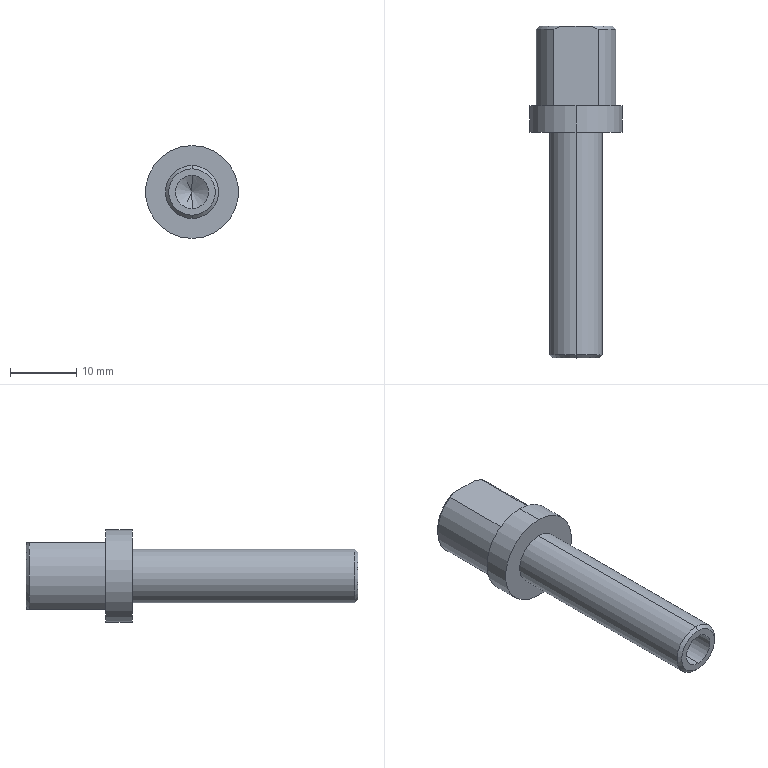Part | SolidWorks | features ICE 3, Chamfer 2, HoleWzd 2, MoveFace 2, Extrusion 1, Revolution 1 | 1 solid | 27 faces | box 14 x 50 x 14 mm | volume 2981 mm3 | cylinder 12 | cone 8 | plane 7 | commonest cylinder face diameters 5 x4 4 x2 8 x2 12 x2 14 x2
STEP:
#1=CARTESIAN_POINT('',(0.,-48.5,4.));
#2=VERTEX_POINT('',#1);
#3=CARTESIAN_POINT('',(0.,-48.5,-4.));
#4=VERTEX_POINT('',#3);
#5=CARTESIAN_POINT('',(0.,-48.5,0.));
#6=DIRECTION('',(0.,1.,0.));
#7=DIRECTION('',(0.,0.,-1.));
#8=AXIS2_PLACEMENT_3D('',#5,#6,#7);
#9=CIRCLE('',#8,4.);
#10=EDGE_CURVE('',#2,#4,#9,.T.);
#11=ORIENTED_EDGE('',*,*,#10,.T.);
#12=CARTESIAN_POINT('',(0.,-15.,-4.));
#13=VERTEX_POINT('',#12);
#14=CARTESIAN_POINT('',(0.,-49.,-4.));
#15=DIRECTION('',(0.,1.,0.));
#16=VECTOR('',#15,1000.);
#17=LINE('',#14,#16);
#18=EDGE_CURVE('',#4,#13,#17,.T.);
#19=ORIENTED_EDGE('',*,*,#18,.T.);
#20=CARTESIAN_POINT('',(0.,-15.,4.));
#21=VERTEX_POINT('',#20);
#22=CARTESIAN_POINT('',(0.,-15.,0.));
#23=DIRECTION('',(0.,1.,0.));
#24=DIRECTION('',(0.,0.,1.));
#25=AXIS2_PLACEMENT_3D('',#22,#23,#24);
#26=CIRCLE('',#25,4.);
#27=EDGE_CURVE('',#21,#13,#26,.T.);
#28=ORIENTED_EDGE('',*,*,#27,.F.);
#29=CARTESIAN_POINT('',(0.,-49.,4.));
#30=DIRECTION('',(0.,1.,0.));
#31=VECTOR('',#30,1000.);
#32=LINE('',#29,#31);
#33=EDGE_CURVE('',#2,#21,#32,.T.);
#34=ORIENTED_EDGE('',*,*,#33,.F.);
#35=EDGE_LOOP('',(#11,#19,#28,#34));
#36=FACE_OUTER_BOUND('',#35,.T.);
#37=CARTESIAN_POINT('',(0.,-49.,0.));
#38=DIRECTION('',(0.,1.,0.));
#39=DIRECTION('',(0.,0.,1.));
#40=AXIS2_PLACEMENT_3D('',#37,#38,#39);
#41=CYLINDRICAL_SURFACE('',#40,4.);
#42=ADVANCED_FACE('',(#36),#41,.T.);
#43=CARTESIAN_POINT('',(0.,-49.,-3.5));
#44=VERTEX_POINT('',#43);
#45=CARTESIAN_POINT('',(0.,-49.,3.5));
#46=VERTEX_POINT('',#45);
#47=CARTESIAN_POINT('',(0.,-49.,0.));
#48=DIRECTION('',(0.,-1.,0.));
#49=DIRECTION('',(0.,0.,-1.));
#50=AXIS2_PLACEMENT_3D('',#47,#48,#49);
#51=CIRCLE('',#50,3.5);
#52=EDGE_CURVE('',#44,#46,#51,.T.);
#53=ORIENTED_EDGE('',*,*,#52,.F.);
#54=CARTESIAN_POINT('',(0.,-49.,-3.5));
#55=DIRECTION('',(0.,0.7071,-0.7071));
#56=VECTOR('',#55,1000.);
#57=LINE('',#54,#56);
#58=EDGE_CURVE('',#44,#4,#57,.T.);
#59=ORIENTED_EDGE('',*,*,#58,.T.);
#60=ORIENTED_EDGE('',*,*,#10,.F.);
#61=CARTESIAN_POINT('',(0.,-49.,3.5));
#62=DIRECTION('',(0.,0.7071,0.7071));
#63=VECTOR('',#62,1000.);
#64=LINE('',#61,#63);
#65=EDGE_CURVE('',#46,#2,#64,.T.);
#66=ORIENTED_EDGE('',*,*,#65,.F.);
#67=EDGE_LOOP('',(#53,#59,#60,#66));
#68=FACE_OUTER_BOUND('',#67,.T.);
#69=CARTESIAN_POINT('',(0.,-49.,0.));
#70=DIRECTION('',(0.,1.,0.));
#71=DIRECTION('',(0.,0.,1.));
#72=AXIS2_PLACEMENT_3D('',#69,#70,#71);
#73=CONICAL_SURFACE('',#72,3.5,0.7854);
#74=ADVANCED_FACE('',(#68),#73,.T.);
#75=CARTESIAN_POINT('',(0.,-34.,2.5));
#76=VERTEX_POINT('',#75);
#77=CARTESIAN_POINT('',(0.,-34.,-2.5));
#78=VERTEX_POINT('',#77);
#79=CARTESIAN_POINT('',(0.,-34.,0.));
#80=DIRECTION('',(0.,-1.,0.));
#81=DIRECTION('',(0.,0.,-1.));
#82=AXIS2_PLACEMENT_3D('',#79,#80,#81);
#83=CIRCLE('',#82,2.5);
#84=EDGE_CURVE('',#76,#78,#83,.T.);
#85=ORIENTED_EDGE('',*,*,#84,.F.);
#86=CARTESIAN_POINT('',(0.,-49.,2.5));
#87=VERTEX_POINT('',#86);
#88=CARTESIAN_POINT('',(0.,-49.,2.5));
#89=DIRECTION('',(0.,-1.,0.));
#90=VECTOR('',#89,1000.);
#91=LINE('',#88,#90);
#92=EDGE_CURVE('',#76,#87,#91,.T.);
#93=ORIENTED_EDGE('',*,*,#92,.T.);
#94=CARTESIAN_POINT('',(0.,-49.,-2.5));
#95=VERTEX_POINT('',#94);
#96=CARTESIAN_POINT('',(0.,-49.,0.));
#97=DIRECTION('',(0.,-1.,0.));
#98=DIRECTION('',(0.,0.,-1.));
#99=AXIS2_PLACEMENT_3D('',#96,#97,#98);
#100=CIRCLE('',#99,2.5);
#101=EDGE_CURVE('',#87,#95,#100,.T.);
#102=ORIENTED_EDGE('',*,*,#101,.T.);
#103=CARTESIAN_POINT('',(0.,-49.,-2.5));
#104=DIRECTION('',(0.,-1.,0.));
#105=VECTOR('',#104,1000.);
#106=LINE('',#103,#105);
#107=EDGE_CURVE('',#78,#95,#106,.T.);
#108=ORIENTED_EDGE('',*,*,#107,.F.);
#109=EDGE_LOOP('',(#85,#93,#102,#108));
#110=FACE_OUTER_BOUND('',#109,.T.);
#111=CARTESIAN_POINT('',(0.,-49.,0.));
#112=DIRECTION('',(0.,-1.,0.));
#113=DIRECTION('',(0.,0.,-1.));
#114=AXIS2_PLACEMENT_3D('',#111,#112,#113);
#115=CYLINDRICAL_SURFACE('',#114,2.5);
#116=ADVANCED_FACE('',(#110),#115,.F.);
#117=CARTESIAN_POINT('',(0.,-32.498,0.));
#118=VERTEX_POINT('',#117);
#119=CARTESIAN_POINT('',(0.,-34.,-2.5));
#120=DIRECTION('',(0.,-0.515,-0.8572));
#121=VECTOR('',#120,1000.);
#122=LINE('',#119,#121);
#123=EDGE_CURVE('',#118,#78,#122,.T.);
#124=ORIENTED_EDGE('',*,*,#123,.F.);
#125=CARTESIAN_POINT('',(0.,-34.,2.5));
#126=DIRECTION('',(0.,-0.515,0.8572));
#127=VECTOR('',#126,1000.);
#128=LINE('',#125,#127);
#129=EDGE_CURVE('',#118,#76,#128,.T.);
#130=ORIENTED_EDGE('',*,*,#129,.T.);
#131=ORIENTED_EDGE('',*,*,#84,.T.);
#132=EDGE_LOOP('',(#124,#130,#131));
#133=FACE_OUTER_BOUND('',#132,.T.);
#134=CARTESIAN_POINT('',(0.,-34.,0.));
#135=DIRECTION('',(0.,-1.,0.));
#136=DIRECTION('',(0.,0.,-1.));
#137=AXIS2_PLACEMENT_3D('',#134,#135,#136);
#138=CONICAL_SURFACE('',#137,2.5,1.03);
#139=ADVANCED_FACE('',(#133),#138,.F.);
#140=CARTESIAN_POINT('',(0.,-15.,-7.));
#141=VERTEX_POINT('',#140);
#142=CARTESIAN_POINT('',(0.,-15.,7.));
#143=VERTEX_POINT('',#142);
#144=CARTESIAN_POINT('',(0.,-15.,0.));
#145=DIRECTION('',(0.,-1.,0.));
#146=DIRECTION('',(0.,0.,1.));
#147=AXIS2_PLACEMENT_3D('',#144,#145,#146);
#148=CIRCLE('',#147,7.);
#149=EDGE_CURVE('',#141,#143,#148,.T.);
#150=ORIENTED_EDGE('',*,*,#149,.F.);
#151=CARTESIAN_POINT('',(0.,-11.,-7.));
#152=VERTEX_POINT('',#151);
#153=CARTESIAN_POINT('',(0.,0.,-7.));
#154=DIRECTION('',(0.,1.,0.));
#155=VECTOR('',#154,1000.);
#156=LINE('',#153,#155);
#157=EDGE_CURVE('',#141,#152,#156,.T.);
#158=ORIENTED_EDGE('',*,*,#157,.T.);
#159=CARTESIAN_POINT('',(0.,-11.,7.));
#160=VERTEX_POINT('',#159);
#161=CARTESIAN_POINT('',(0.,-11.,0.));
#162=DIRECTION('',(0.,1.,0.));
#163=DIRECTION('',(0.,0.,1.));
#164=AXIS2_PLACEMENT_3D('',#161,#162,#163);
#165=CIRCLE('',#164,7.);
#166=EDGE_CURVE('',#160,#152,#165,.T.);
#167=ORIENTED_EDGE('',*,*,#166,.F.);
#168=CARTESIAN_POINT('',(0.,0.,7.));
#169=DIRECTION('',(0.,1.,0.));
#170=VECTOR('',#169,1000.);
#171=LINE('',#168,#170);
#172=EDGE_CURVE('',#143,#160,#171,.T.);
#173=ORIENTED_EDGE('',*,*,#172,.F.);
#174=EDGE_LOOP('',(#150,#158,#167,#173));
#175=FACE_OUTER_BOUND('',#174,.T.);
#176=CARTESIAN_POINT('',(0.,0.,0.));
#177=DIRECTION('',(0.,1.,0.));
#178=DIRECTION('',(0.,0.,1.));
#179=AXIS2_PLACEMENT_3D('',#176,#177,#178);
#180=CYLINDRICAL_SURFACE('',#179,7.);
#181=ADVANCED_FACE('',(#175),#180,.T.);
#182=CARTESIAN_POINT('',(0.,-15.502,0.));
#183=VERTEX_POINT('',#182);
#184=CARTESIAN_POINT('',(0.,-14.3,2.));
#185=VERTEX_POINT('',#184);
#186=CARTESIAN_POINT('',(0.,-14.,2.5));
#187=DIRECTION('',(0.,0.515,0.8572));
#188=VECTOR('',#187,1000.);
#189=LINE('',#186,#188);
#190=EDGE_CURVE('',#183,#185,#189,.T.);
#191=ORIENTED_EDGE('',*,*,#190,.F.);
#192=CARTESIAN_POINT('',(0.,-14.3,-2.));
#193=VERTEX_POINT('',#192);
#194=CARTESIAN_POINT('',(0.,-14.,-2.5));
#195=DIRECTION('',(0.,0.515,-0.8572));
#196=VECTOR('',#195,1000.);
#197=LINE('',#194,#196);
#198=EDGE_CURVE('',#183,#193,#197,.T.);
#199=ORIENTED_EDGE('',*,*,#198,.T.);
#200=CARTESIAN_POINT('',(0.,-14.3,0.));
#201=DIRECTION('',(0.,-1.,0.));
#202=DIRECTION('',(0.,0.,1.));
#203=AXIS2_PLACEMENT_3D('',#200,#201,#202);
#204=CIRCLE('',#203,2.);
#205=EDGE_CURVE('',#185,#193,#204,.T.);
#206=ORIENTED_EDGE('',*,*,#205,.F.);
#207=EDGE_LOOP('',(#191,#199,#206));
#208=FACE_OUTER_BOUND('',#207,.T.);
#209=CARTESIAN_POINT('',(0.,-14.,0.));
#210=DIRECTION('',(0.,1.,0.));
#211=DIRECTION('',(0.,0.,1.));
#212=AXIS2_PLACEMENT_3D('',#209,#210,#211);
#213=CONICAL_SURFACE('',#212,2.5,1.03);
#214=ADVANCED_FACE('',(#208),#213,.F.);
#215=ORIENTED_EDGE('',*,*,#205,.T.);
#216=CARTESIAN_POINT('',(0.,-11.,-2.));
#217=VERTEX_POINT('',#216);
#218=CARTESIAN_POINT('',(0.,0.,-2.));
#219=DIRECTION('',(0.,1.,0.));
#220=VECTOR('',#219,1000.);
#221=LINE('',#218,#220);
#222=EDGE_CURVE('',#193,#217,#221,.T.);
#223=ORIENTED_EDGE('',*,*,#222,.T.);
#224=CARTESIAN_POINT('',(0.,-11.,2.));
#225=VERTEX_POINT('',#224);
#226=CARTESIAN_POINT('',(0.,-11.,0.));
#227=DIRECTION('',(0.,1.,0.));
#228=DIRECTION('',(0.,0.,1.));
#229=AXIS2_PLACEMENT_3D('',#226,#227,#228);
#230=CIRCLE('',#229,2.);
#231=EDGE_CURVE('',#217,#225,#230,.T.);
#232=ORIENTED_EDGE('',*,*,#231,.T.);
#233=CARTESIAN_POINT('',(0.,0.,2.));
#234=DIRECTION('',(0.,1.,0.));
#235=VECTOR('',#234,1000.);
#236=LINE('',#233,#235);
#237=EDGE_CURVE('',#185,#225,#236,.T.);
#238=ORIENTED_EDGE('',*,*,#237,.F.);
#239=EDGE_LOOP('',(#215,#223,#232,#238));
#240=FACE_OUTER_BOUND('',#239,.T.);
#241=CARTESIAN_POINT('',(0.,0.,0.));
#242=DIRECTION('',(0.,1.,0.));
#243=DIRECTION('',(0.,0.,1.));
#244=AXIS2_PLACEMENT_3D('',#241,#242,#243);
#245=CYLINDRICAL_SURFACE('',#244,2.);
#246=ADVANCED_FACE('',(#240),#245,.F.);
#247=CARTESIAN_POINT('',(0.,-11.,-2.5));
#248=VERTEX_POINT('',#247);
#249=CARTESIAN_POINT('',(0.,-11.,2.5));
#250=VERTEX_POINT('',#249);
#251=CARTESIAN_POINT('',(0.,-11.,0.));
#252=DIRECTION('',(0.,1.,0.));
#253=DIRECTION('',(0.,0.,-1.));
#254=AXIS2_PLACEMENT_3D('',#251,#252,#253);
#255=CIRCLE('',#254,2.5);
#256=EDGE_CURVE('',#248,#250,#255,.T.);
#257=ORIENTED_EDGE('',*,*,#256,.F.);
#258=CARTESIAN_POINT('',(0.,1.,-2.5));
#259=VERTEX_POINT('',#258);
#260=CARTESIAN_POINT('',(0.,1.,-2.5));
#261=DIRECTION('',(0.,1.,0.));
#262=VECTOR('',#261,1000.);
#263=LINE('',#260,#262);
#264=EDGE_CURVE('',#248,#259,#263,.T.);
#265=ORIENTED_EDGE('',*,*,#264,.T.);
#266=CARTESIAN_POINT('',(0.,1.,2.5));
#267=VERTEX_POINT('',#266);
#268=CARTESIAN_POINT('',(0.,1.,0.));
#269=DIRECTION('',(0.,1.,0.));
#270=DIRECTION('',(0.,0.,1.));
#271=AXIS2_PLACEMENT_3D('',#268,#269,#270);
#272=CIRCLE('',#271,2.5);
#273=EDGE_CURVE('',#259,#267,#272,.T.);
#274=ORIENTED_EDGE('',*,*,#273,.T.);
#275=CARTESIAN_POINT('',(0.,1.,2.5));
#276=DIRECTION('',(0.,1.,0.));
#277=VECTOR('',#276,1000.);
#278=LINE('',#275,#277);
#279=EDGE_CURVE('',#250,#267,#278,.T.);
#280=ORIENTED_EDGE('',*,*,#279,.F.);
#281=EDGE_LOOP('',(#257,#265,#274,#280));
#282=FACE_OUTER_BOUND('',#281,.T.);
#283=CARTESIAN_POINT('',(0.,1.,0.));
#284=DIRECTION('',(0.,1.,0.));
#285=DIRECTION('',(0.,0.,1.));
#286=AXIS2_PLACEMENT_3D('',#283,#284,#285);
#287=CYLINDRICAL_SURFACE('',#286,2.5);
#288=ADVANCED_FACE('',(#282),#287,.F.);
#289=CARTESIAN_POINT('',(-3.317,0.5,-5.));
#290=VERTEX_POINT('',#289);
#291=CARTESIAN_POINT('',(-2.291,1.,-5.));
#292=VERTEX_POINT('',#291);
#293=CARTESIAN_POINT('',(-3.317,0.5,-5.));
#294=CARTESIAN_POINT('',(-2.983,0.6843,-5.));
#295=CARTESIAN_POINT('',(-2.643,0.8536,-5.));
#296=CARTESIAN_POINT('',(-2.291,1.,-5.));
#297=B_SPLINE_CURVE_WITH_KNOTS('',3,(#293,#294,#295,#296),.UNSPECIFIED.,.F.,.F.,(4,4),(0.01129,0.01243),.UNSPECIFIED.);
#298=EDGE_CURVE('',#290,#292,#297,.T.);
#299=ORIENTED_EDGE('',*,*,#298,.F.);
#300=CARTESIAN_POINT('',(-3.317,0.5,5.));
#301=VERTEX_POINT('',#300);
#302=CARTESIAN_POINT('',(0.,0.5,0.));
#303=DIRECTION('',(0.,-1.,0.));
#304=DIRECTION('',(0.,0.,1.));
#305=AXIS2_PLACEMENT_3D('',#302,#303,#304);
#306=CIRCLE('',#305,6.);
#307=EDGE_CURVE('',#301,#290,#306,.T.);
#308=ORIENTED_EDGE('',*,*,#307,.F.);
#309=CARTESIAN_POINT('',(-2.291,1.,5.));
#310=VERTEX_POINT('',#309);
#311=CARTESIAN_POINT('',(-2.291,1.,5.));
#312=CARTESIAN_POINT('',(-2.644,0.8529,5.));
#313=CARTESIAN_POINT('',(-2.985,0.6835,5.));
#314=CARTESIAN_POINT('',(-3.317,0.5,5.));
#315=B_SPLINE_CURVE_WITH_KNOTS('',3,(#311,#312,#313,#314),.UNSPECIFIED.,.F.,.F.,(4,4),(0.01715,0.0183),.UNSPECIFIED.);
#316=EDGE_CURVE('',#310,#301,#315,.T.);
#317=ORIENTED_EDGE('',*,*,#316,.F.);
#318=CARTESIAN_POINT('',(0.,1.,0.));
#319=DIRECTION('',(0.,1.,0.));
#320=DIRECTION('',(0.,0.,1.));
#321=AXIS2_PLACEMENT_3D('',#318,#319,#320);
#322=CIRCLE('',#321,5.5);
#323=EDGE_CURVE('',#292,#310,#322,.T.);
#324=ORIENTED_EDGE('',*,*,#323,.F.);
#325=EDGE_LOOP('',(#299,#308,#317,#324));
#326=FACE_OUTER_BOUND('',#325,.T.);
#327=CARTESIAN_POINT('',(0.,1.,0.));
#328=DIRECTION('',(0.,-1.,0.));
#329=DIRECTION('',(0.,0.,-1.));
#330=AXIS2_PLACEMENT_3D('',#327,#328,#329);
#331=CONICAL_SURFACE('',#330,5.5,0.7854);
#332=ADVANCED_FACE('',(#326),#331,.T.);
#333=ORIENTED_EDGE('',*,*,#307,.T.);
#334=CARTESIAN_POINT('',(-3.317,-11.,-5.));
#335=VERTEX_POINT('',#334);
#336=CARTESIAN_POINT('',(-3.317,1.,-5.));
#337=DIRECTION('',(0.,-1.,0.));
#338=VECTOR('',#337,1000.);
#339=LINE('',#336,#338);
#340=EDGE_CURVE('',#290,#335,#339,.T.);
#341=ORIENTED_EDGE('',*,*,#340,.T.);
#342=CARTESIAN_POINT('',(-3.317,-11.,5.));
#343=VERTEX_POINT('',#342);
#344=CARTESIAN_POINT('',(0.,-11.,0.));
#345=DIRECTION('',(0.,-1.,0.));
#346=DIRECTION('',(0.,0.,-1.));
#347=AXIS2_PLACEMENT_3D('',#344,#345,#346);
#348=CIRCLE('',#347,6.);
#349=EDGE_CURVE('',#343,#335,#348,.T.);
#350=ORIENTED_EDGE('',*,*,#349,.F.);
#351=CARTESIAN_POINT('',(-3.317,1.,5.));
#352=DIRECTION('',(0.,1.,0.));
#353=VECTOR('',#352,1000.);
#354=LINE('',#351,#353);
#355=EDGE_CURVE('',#343,#301,#354,.T.);
#356=ORIENTED_EDGE('',*,*,#355,.T.);
#357=EDGE_LOOP('',(#333,#341,#350,#356));
#358=FACE_OUTER_BOUND('',#357,.T.);
#359=CARTESIAN_POINT('',(0.,1.,0.));
#360=DIRECTION('',(0.,-1.,0.));
#361=DIRECTION('',(0.,0.,-1.));
#362=AXIS2_PLACEMENT_3D('',#359,#360,#361);
#363=CYLINDRICAL_SURFACE('',#362,6.);
#364=ADVANCED_FACE('',(#358),#363,.T.);
#365=CARTESIAN_POINT('',(3.317,-11.,5.));
#366=VERTEX_POINT('',#365);
#367=CARTESIAN_POINT('',(-8.996,-11.,5.));
#368=DIRECTION('',(1.,0.,0.));
#369=VECTOR('',#368,1000.);
#370=LINE('',#367,#369);
#371=EDGE_CURVE('',#343,#366,#370,.T.);
#372=ORIENTED_EDGE('',*,*,#371,.F.);
#373=ORIENTED_EDGE('',*,*,#349,.T.);
#374=CARTESIAN_POINT('',(3.317,-11.,-5.));
#375=VERTEX_POINT('',#374);
#376=CARTESIAN_POINT('',(-8.996,-11.,-5.));
#377=DIRECTION('',(-1.,0.,0.));
#378=VECTOR('',#377,1000.);
#379=LINE('',#376,#378);
#380=EDGE_CURVE('',#375,#335,#379,.T.);
#381=ORIENTED_EDGE('',*,*,#380,.F.);
#382=CARTESIAN_POINT('',(0.,-11.,0.));
#383=DIRECTION('',(0.,-1.,0.));
#384=DIRECTION('',(0.,0.,-1.));
#385=AXIS2_PLACEMENT_3D('',#382,#383,#384);
#386=CIRCLE('',#385,6.);
#387=EDGE_CURVE('',#375,#366,#386,.T.);
#388=ORIENTED_EDGE('',*,*,#387,.T.);
#389=EDGE_LOOP('',(#372,#373,#381,#388));
#390=FACE_BOUND('',#389,.T.);
#391=ORIENTED_EDGE('',*,*,#166,.T.);
#392=CARTESIAN_POINT('',(0.,-11.,0.));
#393=DIRECTION('',(0.,1.,0.));
#394=DIRECTION('',(0.,0.,1.));
#395=AXIS2_PLACEMENT_3D('',#392,#393,#394);
#396=CIRCLE('',#395,7.);
#397=EDGE_CURVE('',#152,#160,#396,.T.);
#398=ORIENTED_EDGE('',*,*,#397,.T.);
#399=EDGE_LOOP('',(#391,#398));
#400=FACE_OUTER_BOUND('',#399,.T.);
#401=CARTESIAN_POINT('',(0.,-11.,-7.));
#402=DIRECTION('',(0.,-1.,0.));
#403=DIRECTION('',(0.,0.,-1.));
#404=AXIS2_PLACEMENT_3D('',#401,#402,#403);
#405=PLANE('',#404);
#406=ADVANCED_FACE('',(#390,#400),#405,.F.);
#407=CARTESIAN_POINT('',(2.291,1.,-5.));
#408=VERTEX_POINT('',#407);
#409=CARTESIAN_POINT('',(3.317,0.5,-5.));
#410=VERTEX_POINT('',#409);
#411=CARTESIAN_POINT('',(2.291,1.,-5.));
#412=CARTESIAN_POINT('',(2.644,0.8529,-5.));
#413=CARTESIAN_POINT('',(2.985,0.6835,-5.));
#414=CARTESIAN_POINT('',(3.317,0.5,-5.));
#415=B_SPLINE_CURVE_WITH_KNOTS('',3,(#411,#412,#413,#414),.UNSPECIFIED.,.F.,.F.,(4,4),(0.01715,0.0183),.UNSPECIFIED.);
#416=EDGE_CURVE('',#408,#410,#415,.T.);
#417=ORIENTED_EDGE('',*,*,#416,.F.);
#418=CARTESIAN_POINT('',(2.291,1.,5.));
#419=VERTEX_POINT('',#418);
#420=CARTESIAN_POINT('',(0.,1.,0.));
#421=DIRECTION('',(0.,1.,0.));
#422=DIRECTION('',(0.,0.,1.));
#423=AXIS2_PLACEMENT_3D('',#420,#421,#422);
#424=CIRCLE('',#423,5.5);
#425=EDGE_CURVE('',#419,#408,#424,.T.);
#426=ORIENTED_EDGE('',*,*,#425,.F.);
#427=CARTESIAN_POINT('',(3.317,0.5,5.));
#428=VERTEX_POINT('',#427);
#429=CARTESIAN_POINT('',(3.317,0.5,5.));
#430=CARTESIAN_POINT('',(2.983,0.6843,5.));
#431=CARTESIAN_POINT('',(2.643,0.8536,5.));
#432=CARTESIAN_POINT('',(2.291,1.,5.));
#433=B_SPLINE_CURVE_WITH_KNOTS('',3,(#429,#430,#431,#432),.UNSPECIFIED.,.F.,.F.,(4,4),(0.01129,0.01243),.UNSPECIFIED.);
#434=EDGE_CURVE('',#428,#419,#433,.T.);
#435=ORIENTED_EDGE('',*,*,#434,.F.);
#436=CARTESIAN_POINT('',(0.,0.5,0.));
#437=DIRECTION('',(0.,-1.,0.));
#438=DIRECTION('',(0.,0.,1.));
#439=AXIS2_PLACEMENT_3D('',#436,#437,#438);
#440=CIRCLE('',#439,6.);
#441=EDGE_CURVE('',#410,#428,#440,.T.);
#442=ORIENTED_EDGE('',*,*,#441,.F.);
#443=EDGE_LOOP('',(#417,#426,#435,#442));
#444=FACE_OUTER_BOUND('',#443,.T.);
#445=CARTESIAN_POINT('',(0.,1.,0.));
#446=DIRECTION('',(0.,-1.,0.));
#447=DIRECTION('',(0.,0.,-1.));
#448=AXIS2_PLACEMENT_3D('',#445,#446,#447);
#449=CONICAL_SURFACE('',#448,5.5,0.7854);
#450=ADVANCED_FACE('',(#444),#449,.T.);
#451=CARTESIAN_POINT('',(-8.996,1.,-5.));
#452=DIRECTION('',(1.,0.,0.));
#453=VECTOR('',#452,1000.);
#454=LINE('',#451,#453);
#455=EDGE_CURVE('',#292,#408,#454,.T.);
#456=ORIENTED_EDGE('',*,*,#455,.F.);
#457=ORIENTED_EDGE('',*,*,#323,.T.);
#458=CARTESIAN_POINT('',(-8.996,1.,5.));
#459=DIRECTION('',(-1.,0.,0.));
#460=VECTOR('',#459,1000.);
#461=LINE('',#458,#460);
#462=EDGE_CURVE('',#419,#310,#461,.T.);
#463=ORIENTED_EDGE('',*,*,#462,.F.);
#464=ORIENTED_EDGE('',*,*,#425,.T.);
#465=EDGE_LOOP('',(#456,#457,#463,#464));
#466=FACE_OUTER_BOUND('',#465,.T.);
#467=CARTESIAN_POINT('',(0.,1.,0.));
#468=DIRECTION('',(0.,1.,0.));
#469=DIRECTION('',(0.,0.,1.));
#470=AXIS2_PLACEMENT_3D('',#467,#468,#469);
#471=CIRCLE('',#470,2.5);
#472=EDGE_CURVE('',#267,#259,#471,.T.);
#473=ORIENTED_EDGE('',*,*,#472,.F.);
#474=ORIENTED_EDGE('',*,*,#273,.F.);
#475=EDGE_LOOP('',(#473,#474));
#476=FACE_BOUND('',#475,.T.);
#477=CARTESIAN_POINT('',(0.,1.,0.));
#478=DIRECTION('',(0.,1.,0.));
#479=DIRECTION('',(0.,0.,1.));
#480=AXIS2_PLACEMENT_3D('',#477,#478,#479);
#481=PLANE('',#480);
#482=ADVANCED_FACE('',(#466,#476),#481,.T.);
#483=ORIENTED_EDGE('',*,*,#264,.F.);
#484=CARTESIAN_POINT('',(0.,-11.,0.));
#485=DIRECTION('',(0.,1.,0.));
#486=DIRECTION('',(0.,0.,-1.));
#487=AXIS2_PLACEMENT_3D('',#484,#485,#486);
#488=CIRCLE('',#487,2.5);
#489=EDGE_CURVE('',#250,#248,#488,.T.);
#490=ORIENTED_EDGE('',*,*,#489,.F.);
#491=ORIENTED_EDGE('',*,*,#279,.T.);
#492=ORIENTED_EDGE('',*,*,#472,.T.);
#493=EDGE_LOOP('',(#483,#490,#491,#492));
#494=FACE_OUTER_BOUND('',#493,.T.);
#495=CARTESIAN_POINT('',(0.,1.,0.));
#496=DIRECTION('',(0.,1.,0.));
#497=DIRECTION('',(0.,0.,1.));
#498=AXIS2_PLACEMENT_3D('',#495,#496,#497);
#499=CYLINDRICAL_SURFACE('',#498,2.5);
#500=ADVANCED_FACE('',(#494),#499,.F.);
#501=ORIENTED_EDGE('',*,*,#387,.F.);
#502=CARTESIAN_POINT('',(3.317,1.,-5.));
#503=DIRECTION('',(0.,1.,0.));
#504=VECTOR('',#503,1000.);
#505=LINE('',#502,#504);
#506=EDGE_CURVE('',#375,#410,#505,.T.);
#507=ORIENTED_EDGE('',*,*,#506,.T.);
#508=ORIENTED_EDGE('',*,*,#441,.T.);
#509=CARTESIAN_POINT('',(3.317,1.,5.));
#510=DIRECTION('',(0.,-1.,0.));
#511=VECTOR('',#510,1000.);
#512=LINE('',#509,#511);
#513=EDGE_CURVE('',#428,#366,#512,.T.);
#514=ORIENTED_EDGE('',*,*,#513,.T.);
#515=EDGE_LOOP('',(#501,#507,#508,#514));
#516=FACE_OUTER_BOUND('',#515,.T.);
#517=CARTESIAN_POINT('',(0.,1.,0.));
#518=DIRECTION('',(0.,-1.,0.));
#519=DIRECTION('',(0.,0.,-1.));
#520=AXIS2_PLACEMENT_3D('',#517,#518,#519);
#521=CYLINDRICAL_SURFACE('',#520,6.);
#522=ADVANCED_FACE('',(#516),#521,.T.);
#523=CARTESIAN_POINT('',(0.,-11.,0.));
#524=DIRECTION('',(0.,1.,0.));
#525=DIRECTION('',(0.,0.,1.));
#526=AXIS2_PLACEMENT_3D('',#523,#524,#525);
#527=CIRCLE('',#526,2.);
#528=EDGE_CURVE('',#225,#217,#527,.T.);
#529=ORIENTED_EDGE('',*,*,#528,.F.);
#530=ORIENTED_EDGE('',*,*,#231,.F.);
#531=EDGE_LOOP('',(#529,#530));
#532=FACE_BOUND('',#531,.T.);
#533=ORIENTED_EDGE('',*,*,#489,.T.);
#534=ORIENTED_EDGE('',*,*,#256,.T.);
#535=EDGE_LOOP('',(#533,#534));
#536=FACE_OUTER_BOUND('',#535,.T.);
#537=CARTESIAN_POINT('',(0.,-11.,-7.));
#538=DIRECTION('',(0.,-1.,0.));
#539=DIRECTION('',(0.,0.,-1.));
#540=AXIS2_PLACEMENT_3D('',#537,#538,#539);
#541=PLANE('',#540);
#542=ADVANCED_FACE('',(#532,#536),#541,.F.);
#543=ORIENTED_EDGE('',*,*,#222,.F.);
#544=CARTESIAN_POINT('',(0.,-14.3,0.));
#545=DIRECTION('',(0.,-1.,0.));
#546=DIRECTION('',(0.,0.,1.));
#547=AXIS2_PLACEMENT_3D('',#544,#545,#546);
#548=CIRCLE('',#547,2.);
#549=EDGE_CURVE('',#193,#185,#548,.T.);
#550=ORIENTED_EDGE('',*,*,#549,.T.);
#551=ORIENTED_EDGE('',*,*,#237,.T.);
#552=ORIENTED_EDGE('',*,*,#528,.T.);
#553=EDGE_LOOP('',(#543,#550,#551,#552));
#554=FACE_OUTER_BOUND('',#553,.T.);
#555=CARTESIAN_POINT('',(0.,0.,0.));
#556=DIRECTION('',(0.,1.,0.));
#557=DIRECTION('',(0.,0.,1.));
#558=AXIS2_PLACEMENT_3D('',#555,#556,#557);
#559=CYLINDRICAL_SURFACE('',#558,2.);
#560=ADVANCED_FACE('',(#554),#559,.F.);
#561=ORIENTED_EDGE('',*,*,#198,.F.);
#562=ORIENTED_EDGE('',*,*,#190,.T.);
#563=ORIENTED_EDGE('',*,*,#549,.F.);
#564=EDGE_LOOP('',(#561,#562,#563));
#565=FACE_OUTER_BOUND('',#564,.T.);
#566=CARTESIAN_POINT('',(0.,-14.,0.));
#567=DIRECTION('',(0.,1.,0.));
#568=DIRECTION('',(0.,0.,1.));
#569=AXIS2_PLACEMENT_3D('',#566,#567,#568);
#570=CONICAL_SURFACE('',#569,2.5,1.03);
#571=ADVANCED_FACE('',(#565),#570,.F.);
#572=ORIENTED_EDGE('',*,*,#355,.F.);
#573=ORIENTED_EDGE('',*,*,#371,.T.);
#574=ORIENTED_EDGE('',*,*,#513,.F.);
#575=ORIENTED_EDGE('',*,*,#434,.T.);
#576=ORIENTED_EDGE('',*,*,#462,.T.);
#577=ORIENTED_EDGE('',*,*,#316,.T.);
#578=EDGE_LOOP('',(#572,#573,#574,#575,#576,#577));
#579=FACE_OUTER_BOUND('',#578,.T.);
#580=CARTESIAN_POINT('',(-8.996,-17.,5.));
#581=DIRECTION('',(0.,0.,-1.));
#582=DIRECTION('',(-1.,0.,0.));
#583=AXIS2_PLACEMENT_3D('',#580,#581,#582);
#584=PLANE('',#583);
#585=ADVANCED_FACE('',(#579),#584,.F.);
#586=ORIENTED_EDGE('',*,*,#506,.F.);
#587=ORIENTED_EDGE('',*,*,#380,.T.);
#588=ORIENTED_EDGE('',*,*,#340,.F.);
#589=ORIENTED_EDGE('',*,*,#298,.T.);
#590=ORIENTED_EDGE('',*,*,#455,.T.);
#591=ORIENTED_EDGE('',*,*,#416,.T.);
#592=EDGE_LOOP('',(#586,#587,#588,#589,#590,#591));
#593=FACE_OUTER_BOUND('',#592,.T.);
#594=CARTESIAN_POINT('',(-8.996,-17.,-5.));
#595=DIRECTION('',(0.,0.,1.));
#596=DIRECTION('',(1.,0.,0.));
#597=AXIS2_PLACEMENT_3D('',#594,#595,#596);
#598=PLANE('',#597);
#599=ADVANCED_FACE('',(#593),#598,.F.);
#600=ORIENTED_EDGE('',*,*,#157,.F.);
#601=CARTESIAN_POINT('',(0.,-15.,0.));
#602=DIRECTION('',(0.,-1.,0.));
#603=DIRECTION('',(0.,0.,1.));
#604=AXIS2_PLACEMENT_3D('',#601,#602,#603);
#605=CIRCLE('',#604,7.);
#606=EDGE_CURVE('',#143,#141,#605,.T.);
#607=ORIENTED_EDGE('',*,*,#606,.F.);
#608=ORIENTED_EDGE('',*,*,#172,.T.);
#609=ORIENTED_EDGE('',*,*,#397,.F.);
#610=EDGE_LOOP('',(#600,#607,#608,#609));
#611=FACE_OUTER_BOUND('',#610,.T.);
#612=CARTESIAN_POINT('',(0.,0.,0.));
#613=DIRECTION('',(0.,1.,0.));
#614=DIRECTION('',(0.,0.,1.));
#615=AXIS2_PLACEMENT_3D('',#612,#613,#614);
#616=CYLINDRICAL_SURFACE('',#615,7.);
#617=ADVANCED_FACE('',(#611),#616,.T.);
#618=ORIENTED_EDGE('',*,*,#129,.F.);
#619=ORIENTED_EDGE('',*,*,#123,.T.);
#620=CARTESIAN_POINT('',(0.,-34.,0.));
#621=DIRECTION('',(0.,-1.,0.));
#622=DIRECTION('',(0.,0.,-1.));
#623=AXIS2_PLACEMENT_3D('',#620,#621,#622);
#624=CIRCLE('',#623,2.5);
#625=EDGE_CURVE('',#78,#76,#624,.T.);
#626=ORIENTED_EDGE('',*,*,#625,.T.);
#627=EDGE_LOOP('',(#618,#619,#626));
#628=FACE_OUTER_BOUND('',#627,.T.);
#629=CARTESIAN_POINT('',(0.,-34.,0.));
#630=DIRECTION('',(0.,-1.,0.));
#631=DIRECTION('',(0.,0.,-1.));
#632=AXIS2_PLACEMENT_3D('',#629,#630,#631);
#633=CONICAL_SURFACE('',#632,2.5,1.03);
#634=ADVANCED_FACE('',(#628),#633,.F.);
#635=ORIENTED_EDGE('',*,*,#92,.F.);
#636=ORIENTED_EDGE('',*,*,#625,.F.);
#637=ORIENTED_EDGE('',*,*,#107,.T.);
#638=CARTESIAN_POINT('',(0.,-49.,0.));
#639=DIRECTION('',(0.,-1.,0.));
#640=DIRECTION('',(0.,0.,-1.));
#641=AXIS2_PLACEMENT_3D('',#638,#639,#640);
#642=CIRCLE('',#641,2.5);
#643=EDGE_CURVE('',#95,#87,#642,.T.);
#644=ORIENTED_EDGE('',*,*,#643,.T.);
#645=EDGE_LOOP('',(#635,#636,#637,#644));
#646=FACE_OUTER_BOUND('',#645,.T.);
#647=CARTESIAN_POINT('',(0.,-49.,0.));
#648=DIRECTION('',(0.,-1.,0.));
#649=DIRECTION('',(0.,0.,-1.));
#650=AXIS2_PLACEMENT_3D('',#647,#648,#649);
#651=CYLINDRICAL_SURFACE('',#650,2.5);
#652=ADVANCED_FACE('',(#646),#651,.F.);
#653=ORIENTED_EDGE('',*,*,#643,.F.);
#654=ORIENTED_EDGE('',*,*,#101,.F.);
#655=EDGE_LOOP('',(#653,#654));
#656=FACE_BOUND('',#655,.T.);
#657=CARTESIAN_POINT('',(0.,-49.,0.));
#658=DIRECTION('',(0.,-1.,0.));
#659=DIRECTION('',(0.,0.,-1.));
#660=AXIS2_PLACEMENT_3D('',#657,#658,#659);
#661=CIRCLE('',#660,3.5);
#662=EDGE_CURVE('',#46,#44,#661,.T.);
#663=ORIENTED_EDGE('',*,*,#662,.T.);
#664=ORIENTED_EDGE('',*,*,#52,.T.);
#665=EDGE_LOOP('',(#663,#664));
#666=FACE_OUTER_BOUND('',#665,.T.);
#667=CARTESIAN_POINT('',(0.,-49.,0.));
#668=DIRECTION('',(0.,-1.,0.));
#669=DIRECTION('',(0.,0.,-1.));
#670=AXIS2_PLACEMENT_3D('',#667,#668,#669);
#671=PLANE('',#670);
#672=ADVANCED_FACE('',(#656,#666),#671,.T.);
#673=ORIENTED_EDGE('',*,*,#58,.F.);
#674=ORIENTED_EDGE('',*,*,#662,.F.);
#675=ORIENTED_EDGE('',*,*,#65,.T.);
#676=CARTESIAN_POINT('',(0.,-48.5,0.));
#677=DIRECTION('',(0.,1.,0.));
#678=DIRECTION('',(0.,0.,-1.));
#679=AXIS2_PLACEMENT_3D('',#676,#677,#678);
#680=CIRCLE('',#679,4.);
#681=EDGE_CURVE('',#4,#2,#680,.T.);
#682=ORIENTED_EDGE('',*,*,#681,.F.);
#683=EDGE_LOOP('',(#673,#674,#675,#682));
#684=FACE_OUTER_BOUND('',#683,.T.);
#685=CARTESIAN_POINT('',(0.,-49.,0.));
#686=DIRECTION('',(0.,1.,0.));
#687=DIRECTION('',(0.,0.,1.));
#688=AXIS2_PLACEMENT_3D('',#685,#686,#687);
#689=CONICAL_SURFACE('',#688,3.5,0.7854);
#690=ADVANCED_FACE('',(#684),#689,.T.);
#691=ORIENTED_EDGE('',*,*,#18,.F.);
#692=ORIENTED_EDGE('',*,*,#681,.T.);
#693=ORIENTED_EDGE('',*,*,#33,.T.);
#694=CARTESIAN_POINT('',(0.,-15.,0.));
#695=DIRECTION('',(0.,1.,0.));
#696=DIRECTION('',(0.,0.,1.));
#697=AXIS2_PLACEMENT_3D('',#694,#695,#696);
#698=CIRCLE('',#697,4.);
#699=EDGE_CURVE('',#13,#21,#698,.T.);
#700=ORIENTED_EDGE('',*,*,#699,.F.);
#701=EDGE_LOOP('',(#691,#692,#693,#700));
#702=FACE_OUTER_BOUND('',#701,.T.);
#703=CARTESIAN_POINT('',(0.,-49.,0.));
#704=DIRECTION('',(0.,1.,0.));
#705=DIRECTION('',(0.,0.,1.));
#706=AXIS2_PLACEMENT_3D('',#703,#704,#705);
#707=CYLINDRICAL_SURFACE('',#706,4.);
#708=ADVANCED_FACE('',(#702),#707,.T.);
#709=ORIENTED_EDGE('',*,*,#27,.T.);
#710=ORIENTED_EDGE('',*,*,#699,.T.);
#711=EDGE_LOOP('',(#709,#710));
#712=FACE_BOUND('',#711,.T.);
#713=ORIENTED_EDGE('',*,*,#606,.T.);
#714=ORIENTED_EDGE('',*,*,#149,.T.);
#715=EDGE_LOOP('',(#713,#714));
#716=FACE_OUTER_BOUND('',#715,.T.);
#717=CARTESIAN_POINT('',(0.,-15.,-7.));
#718=DIRECTION('',(0.,1.,0.));
#719=DIRECTION('',(0.,0.,1.));
#720=AXIS2_PLACEMENT_3D('',#717,#718,#719);
#721=PLANE('',#720);
#722=ADVANCED_FACE('',(#712,#716),#721,.F.);
#723=CLOSED_SHELL('',(#42,#74,#116,#139,#181,#214,#246,#288,#332,#364,#406,#450,#482,#500,#522,#542,#560,#571,#585,#599,#617,#634,#652,#672,#690,#708,#722));
#724=MANIFOLD_SOLID_BREP('',#723);
#725=CARTESIAN_POINT('',(0.,0.,0.));
#726=DIRECTION('',(0.,0.,1.));
#727=DIRECTION('',(1.,0.,0.));
#728=AXIS2_PLACEMENT_3D('',#725,#726,#727);
#729=(LENGTH_UNIT()NAMED_UNIT(*)SI_UNIT(.MILLI.,.METRE.));
#730=UNCERTAINTY_MEASURE_WITH_UNIT(LENGTH_MEASURE(0.00001),#729,'','');
#731=(NAMED_UNIT(*)PLANE_ANGLE_UNIT()SI_UNIT($,.RADIAN.));
#732=(NAMED_UNIT(*)SI_UNIT($,.STERADIAN.)SOLID_ANGLE_UNIT());
#733=(GEOMETRIC_REPRESENTATION_CONTEXT(3)GLOBAL_UNCERTAINTY_ASSIGNED_CONTEXT((#730))GLOBAL_UNIT_ASSIGNED_CONTEXT((#729,#731,#732))REPRESENTATION_CONTEXT('',''));
#734=ADVANCED_BREP_SHAPE_REPRESENTATION('',(#724,#728),#733);